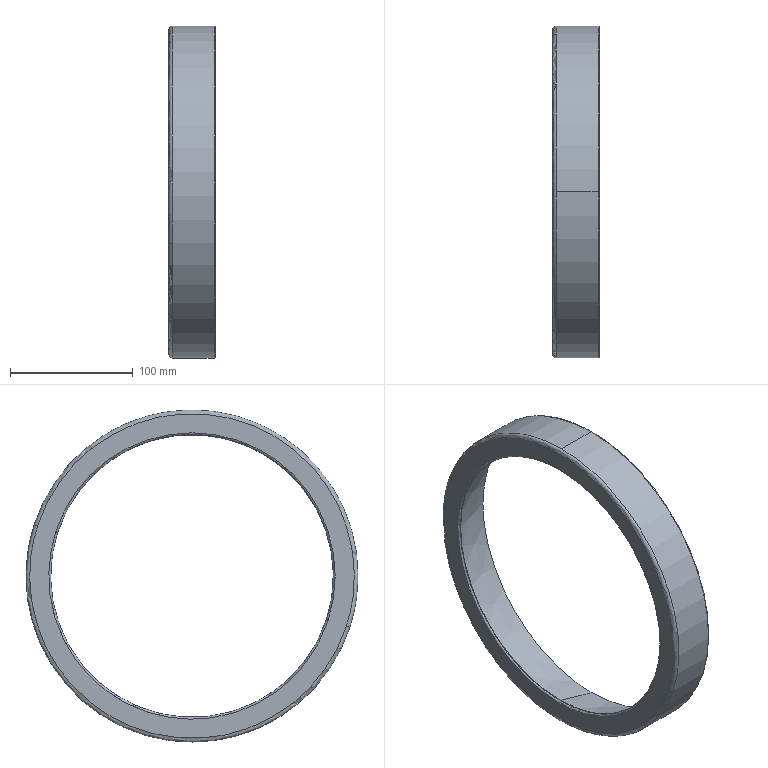Part | SolidWorks | features BaseBody 1 | 1 solid | 14 faces | box 38 x 270 x 270 mm | volume 453986 mm3 | torus 8 | plane 2 | cylinder 2 | cone 2 | commonest cylinder face diameters 270 x2
STEP:
#1=CARTESIAN_POINT('',(0.,-110.751,-35.985));
#2=VERTEX_POINT('',#1);
#3=CARTESIAN_POINT('',(1.5,-109.325,-35.522));
#4=VERTEX_POINT('',#3);
#5=CARTESIAN_POINT('',(1.5,-110.751,-35.985));
#6=DIRECTION('',(0.,0.309,-0.9511));
#7=DIRECTION('',(-1.,0.,0.));
#8=AXIS2_PLACEMENT_3D('',#5,#6,#7);
#9=CIRCLE('',#8,1.5);
#10=EDGE_CURVE('',#2,#4,#9,.T.);
#11=ORIENTED_EDGE('',*,*,#10,.T.);
#12=CARTESIAN_POINT('',(1.5,109.325,35.522));
#13=VERTEX_POINT('',#12);
#14=CARTESIAN_POINT('',(1.5,0.,0.));
#15=DIRECTION('',(1.,0.,0.));
#16=DIRECTION('',(0.,0.,-1.));
#17=AXIS2_PLACEMENT_3D('',#14,#15,#16);
#18=CIRCLE('',#17,114.951);
#19=EDGE_CURVE('',#4,#13,#18,.T.);
#20=ORIENTED_EDGE('',*,*,#19,.T.);
#21=CARTESIAN_POINT('',(0.,110.751,35.985));
#22=VERTEX_POINT('',#21);
#23=CARTESIAN_POINT('',(1.5,110.751,35.985));
#24=DIRECTION('',(0.,-0.309,0.9511));
#25=DIRECTION('',(-1.,0.,0.));
#26=AXIS2_PLACEMENT_3D('',#23,#24,#25);
#27=CIRCLE('',#26,1.5);
#28=EDGE_CURVE('',#22,#13,#27,.T.);
#29=ORIENTED_EDGE('',*,*,#28,.F.);
#30=CARTESIAN_POINT('',(0.,-110.751,-35.985));
#31=CARTESIAN_POINT('',(0.,-108.396,-43.234));
#32=CARTESIAN_POINT('',(0.,-105.327,-50.25));
#33=CARTESIAN_POINT('',(0.,-97.879,-63.55));
#34=CARTESIAN_POINT('',(0.,-93.5,-69.833));
#35=CARTESIAN_POINT('',(0.,-83.6,-81.424));
#36=CARTESIAN_POINT('',(0.,-78.079,-86.732));
#37=CARTESIAN_POINT('',(0.,-66.109,-96.169));
#38=CARTESIAN_POINT('',(0.,-59.659,-100.298));
#39=CARTESIAN_POINT('',(0.,-46.077,-107.219));
#40=CARTESIAN_POINT('',(0.,-38.945,-110.01));
#41=CARTESIAN_POINT('',(0.,-24.274,-114.147));
#42=CARTESIAN_POINT('',(0.,-16.735,-115.494));
#43=CARTESIAN_POINT('',(0.,-1.538,-116.69));
#44=CARTESIAN_POINT('',(0.,6.118,-116.539));
#45=CARTESIAN_POINT('',(0.,21.256,-114.748));
#46=CARTESIAN_POINT('',(0.,28.737,-113.106));
#47=CARTESIAN_POINT('',(0.,43.234,-108.396));
#48=CARTESIAN_POINT('',(0.,50.25,-105.327));
#49=CARTESIAN_POINT('',(0.,63.55,-97.879));
#50=CARTESIAN_POINT('',(0.,69.833,-93.5));
#51=CARTESIAN_POINT('',(0.,81.424,-83.6));
#52=CARTESIAN_POINT('',(0.,86.732,-78.079));
#53=CARTESIAN_POINT('',(0.,96.169,-66.109));
#54=CARTESIAN_POINT('',(0.,100.298,-59.659));
#55=CARTESIAN_POINT('',(0.,107.219,-46.077));
#56=CARTESIAN_POINT('',(0.,110.01,-38.945));
#57=CARTESIAN_POINT('',(0.,114.147,-24.274));
#58=CARTESIAN_POINT('',(0.,115.494,-16.735));
#59=CARTESIAN_POINT('',(0.,116.69,-1.538));
#60=CARTESIAN_POINT('',(0.,116.539,6.118));
#61=CARTESIAN_POINT('',(0.,114.748,21.256));
#62=CARTESIAN_POINT('',(0.,113.106,28.737));
#63=CARTESIAN_POINT('',(0.,110.751,35.985));
#64=B_SPLINE_CURVE_WITH_KNOTS('',3,(#30,#31,#32,#33,#34,#35,#36,#37,#38,#39,#40,#41,#42,#43,#44,#45,#46,#47,#48,#49,#50,#51,#52,#53,#54,#55,#56,#57,#58,#59,#60,#61,#62,#63),.UNSPECIFIED.,.F.,.F.,(4,2,2,2,2,2,2,2,2,2,2,2,2,2,2,2,4),(0.,0.1963,0.3927,0.589,0.7854,0.9817,1.178,1.374,1.571,1.767,1.963,2.16,2.356,2.553,2.749,2.945,3.142),.UNSPECIFIED.);
#65=EDGE_CURVE('',#2,#22,#64,.T.);
#66=ORIENTED_EDGE('',*,*,#65,.F.);
#67=EDGE_LOOP('',(#11,#20,#29,#66));
#68=FACE_OUTER_BOUND('',#67,.T.);
#69=CARTESIAN_POINT('',(1.5,0.,0.));
#70=DIRECTION('',(1.,0.,0.));
#71=DIRECTION('',(0.,-0.309,0.9511));
#72=AXIS2_PLACEMENT_3D('',#69,#70,#71);
#73=TOROIDAL_SURFACE('',#72,116.451,1.5);
#74=ADVANCED_FACE('',(#68),#73,.T.);
#75=ORIENTED_EDGE('',*,*,#28,.T.);
#76=CARTESIAN_POINT('',(1.5,0.,0.));
#77=DIRECTION('',(1.,0.,0.));
#78=DIRECTION('',(0.,0.,-1.));
#79=AXIS2_PLACEMENT_3D('',#76,#77,#78);
#80=CIRCLE('',#79,114.951);
#81=EDGE_CURVE('',#13,#4,#80,.T.);
#82=ORIENTED_EDGE('',*,*,#81,.T.);
#83=ORIENTED_EDGE('',*,*,#10,.F.);
#84=CARTESIAN_POINT('',(0.,0.,0.));
#85=DIRECTION('',(1.,0.,0.));
#86=DIRECTION('',(0.,0.,-1.));
#87=AXIS2_PLACEMENT_3D('',#84,#85,#86);
#88=CIRCLE('',#87,116.451);
#89=EDGE_CURVE('',#22,#2,#88,.T.);
#90=ORIENTED_EDGE('',*,*,#89,.F.);
#91=EDGE_LOOP('',(#75,#82,#83,#90));
#92=FACE_OUTER_BOUND('',#91,.T.);
#93=CARTESIAN_POINT('',(1.5,0.,0.));
#94=DIRECTION('',(1.,0.,0.));
#95=DIRECTION('',(0.,0.309,-0.9511));
#96=AXIS2_PLACEMENT_3D('',#93,#94,#95);
#97=TOROIDAL_SURFACE('',#96,116.451,1.5);
#98=ADVANCED_FACE('',(#92),#97,.T.);
#99=ORIENTED_EDGE('',*,*,#89,.T.);
#100=ORIENTED_EDGE('',*,*,#65,.T.);
#101=EDGE_LOOP('',(#99,#100));
#102=FACE_BOUND('',#101,.T.);
#103=CARTESIAN_POINT('',(0.,125.539,40.79));
#104=VERTEX_POINT('',#103);
#105=CARTESIAN_POINT('',(0.,-125.539,-40.79));
#106=VERTEX_POINT('',#105);
#107=CARTESIAN_POINT('',(0.,125.539,40.79));
#108=CARTESIAN_POINT('',(0.,122.87,49.007));
#109=CARTESIAN_POINT('',(0.,119.391,56.96));
#110=CARTESIAN_POINT('',(0.,110.948,72.036));
#111=CARTESIAN_POINT('',(0.,105.984,79.158));
#112=CARTESIAN_POINT('',(0.,94.763,92.297));
#113=CARTESIAN_POINT('',(0.,88.505,98.313));
#114=CARTESIAN_POINT('',(0.,74.936,109.01));
#115=CARTESIAN_POINT('',(0.,67.624,113.691));
#116=CARTESIAN_POINT('',(0.,52.229,121.535));
#117=CARTESIAN_POINT('',(0.,44.145,124.699));
#118=CARTESIAN_POINT('',(0.,27.515,129.389));
#119=CARTESIAN_POINT('',(0.,18.969,130.915));
#120=CARTESIAN_POINT('',(0.,1.744,132.271));
#121=CARTESIAN_POINT('',(0.,-6.935,132.1));
#122=CARTESIAN_POINT('',(0.,-24.094,130.07));
#123=CARTESIAN_POINT('',(0.,-32.574,128.209));
#124=CARTESIAN_POINT('',(0.,-49.007,122.87));
#125=CARTESIAN_POINT('',(0.,-56.96,119.391));
#126=CARTESIAN_POINT('',(0.,-72.036,110.948));
#127=CARTESIAN_POINT('',(0.,-79.158,105.984));
#128=CARTESIAN_POINT('',(0.,-92.297,94.763));
#129=CARTESIAN_POINT('',(0.,-98.313,88.505));
#130=CARTESIAN_POINT('',(0.,-109.01,74.936));
#131=CARTESIAN_POINT('',(0.,-113.691,67.624));
#132=CARTESIAN_POINT('',(0.,-121.535,52.229));
#133=CARTESIAN_POINT('',(0.,-124.699,44.145));
#134=CARTESIAN_POINT('',(0.,-129.389,27.515));
#135=CARTESIAN_POINT('',(0.,-130.915,18.969));
#136=CARTESIAN_POINT('',(0.,-132.271,1.744));
#137=CARTESIAN_POINT('',(0.,-132.1,-6.935));
#138=CARTESIAN_POINT('',(0.,-130.07,-24.094));
#139=CARTESIAN_POINT('',(0.,-128.209,-32.574));
#140=CARTESIAN_POINT('',(0.,-125.539,-40.79));
#141=B_SPLINE_CURVE_WITH_KNOTS('',3,(#107,#108,#109,#110,#111,#112,#113,#114,#115,#116,#117,#118,#119,#120,#121,#122,#123,#124,#125,#126,#127,#128,#129,#130,#131,#132,#133,#134,#135,#136,#137,#138,#139,#140),.UNSPECIFIED.,.F.,.F.,(4,2,2,2,2,2,2,2,2,2,2,2,2,2,2,2,4),(0.,0.1963,0.3927,0.589,0.7854,0.9817,1.178,1.374,1.571,1.767,1.963,2.16,2.356,2.553,2.749,2.945,3.142),.UNSPECIFIED.);
#142=EDGE_CURVE('',#104,#106,#141,.T.);
#143=ORIENTED_EDGE('',*,*,#142,.F.);
#144=CARTESIAN_POINT('',(0.,-125.539,-40.79));
#145=CARTESIAN_POINT('',(0.,-122.87,-49.007));
#146=CARTESIAN_POINT('',(0.,-119.391,-56.96));
#147=CARTESIAN_POINT('',(0.,-110.948,-72.036));
#148=CARTESIAN_POINT('',(0.,-105.984,-79.158));
#149=CARTESIAN_POINT('',(0.,-94.763,-92.297));
#150=CARTESIAN_POINT('',(0.,-88.505,-98.313));
#151=CARTESIAN_POINT('',(0.,-74.936,-109.01));
#152=CARTESIAN_POINT('',(0.,-67.624,-113.691));
#153=CARTESIAN_POINT('',(0.,-52.229,-121.535));
#154=CARTESIAN_POINT('',(0.,-44.145,-124.699));
#155=CARTESIAN_POINT('',(0.,-27.515,-129.389));
#156=CARTESIAN_POINT('',(0.,-18.969,-130.915));
#157=CARTESIAN_POINT('',(0.,-1.744,-132.271));
#158=CARTESIAN_POINT('',(0.,6.935,-132.1));
#159=CARTESIAN_POINT('',(0.,24.094,-130.07));
#160=CARTESIAN_POINT('',(0.,32.574,-128.209));
#161=CARTESIAN_POINT('',(0.,49.007,-122.87));
#162=CARTESIAN_POINT('',(0.,56.96,-119.391));
#163=CARTESIAN_POINT('',(0.,72.036,-110.948));
#164=CARTESIAN_POINT('',(0.,79.158,-105.984));
#165=CARTESIAN_POINT('',(0.,92.297,-94.763));
#166=CARTESIAN_POINT('',(0.,98.313,-88.505));
#167=CARTESIAN_POINT('',(0.,109.01,-74.936));
#168=CARTESIAN_POINT('',(0.,113.691,-67.624));
#169=CARTESIAN_POINT('',(0.,121.535,-52.229));
#170=CARTESIAN_POINT('',(0.,124.699,-44.145));
#171=CARTESIAN_POINT('',(0.,129.389,-27.515));
#172=CARTESIAN_POINT('',(0.,130.915,-18.969));
#173=CARTESIAN_POINT('',(0.,132.271,-1.744));
#174=CARTESIAN_POINT('',(0.,132.1,6.935));
#175=CARTESIAN_POINT('',(0.,130.07,24.094));
#176=CARTESIAN_POINT('',(0.,128.209,32.574));
#177=CARTESIAN_POINT('',(0.,125.539,40.79));
#178=B_SPLINE_CURVE_WITH_KNOTS('',3,(#144,#145,#146,#147,#148,#149,#150,#151,#152,#153,#154,#155,#156,#157,#158,#159,#160,#161,#162,#163,#164,#165,#166,#167,#168,#169,#170,#171,#172,#173,#174,#175,#176,#177),.UNSPECIFIED.,.F.,.F.,(4,2,2,2,2,2,2,2,2,2,2,2,2,2,2,2,4),(0.,0.1963,0.3927,0.589,0.7854,0.9817,1.178,1.374,1.571,1.767,1.963,2.16,2.356,2.553,2.749,2.945,3.142),.UNSPECIFIED.);
#179=EDGE_CURVE('',#106,#104,#178,.T.);
#180=ORIENTED_EDGE('',*,*,#179,.F.);
#181=EDGE_LOOP('',(#143,#180));
#182=FACE_OUTER_BOUND('',#181,.T.);
#183=CARTESIAN_POINT('',(0.,132.,0.));
#184=DIRECTION('',(-1.,0.,0.));
#185=DIRECTION('',(0.,0.,1.));
#186=AXIS2_PLACEMENT_3D('',#183,#184,#185);
#187=PLANE('',#186);
#188=ADVANCED_FACE('',(#102,#182),#187,.T.);
#189=CARTESIAN_POINT('',(3.,-128.393,-41.717));
#190=VERTEX_POINT('',#189);
#191=CARTESIAN_POINT('',(3.,-125.539,-40.79));
#192=DIRECTION('',(0.,0.309,-0.9511));
#193=DIRECTION('',(0.,-0.9511,-0.309));
#194=AXIS2_PLACEMENT_3D('',#191,#192,#193);
#195=CIRCLE('',#194,3.);
#196=EDGE_CURVE('',#190,#106,#195,.T.);
#197=ORIENTED_EDGE('',*,*,#196,.T.);
#198=ORIENTED_EDGE('',*,*,#179,.T.);
#199=CARTESIAN_POINT('',(3.,128.393,41.717));
#200=VERTEX_POINT('',#199);
#201=CARTESIAN_POINT('',(3.,125.539,40.79));
#202=DIRECTION('',(0.,-0.309,0.9511));
#203=DIRECTION('',(0.,0.9511,0.309));
#204=AXIS2_PLACEMENT_3D('',#201,#202,#203);
#205=CIRCLE('',#204,3.);
#206=EDGE_CURVE('',#200,#104,#205,.T.);
#207=ORIENTED_EDGE('',*,*,#206,.F.);
#208=CARTESIAN_POINT('',(3.,0.,-135.));
#209=VERTEX_POINT('',#208);
#210=CARTESIAN_POINT('',(3.,0.,0.));
#211=DIRECTION('',(1.,0.,0.));
#212=DIRECTION('',(0.,0.,-1.));
#213=AXIS2_PLACEMENT_3D('',#210,#211,#212);
#214=CIRCLE('',#213,135.);
#215=EDGE_CURVE('',#209,#200,#214,.T.);
#216=ORIENTED_EDGE('',*,*,#215,.F.);
#217=CARTESIAN_POINT('',(3.,0.,0.));
#218=DIRECTION('',(1.,0.,0.));
#219=DIRECTION('',(0.,0.,-1.));
#220=AXIS2_PLACEMENT_3D('',#217,#218,#219);
#221=CIRCLE('',#220,135.);
#222=EDGE_CURVE('',#190,#209,#221,.T.);
#223=ORIENTED_EDGE('',*,*,#222,.F.);
#224=EDGE_LOOP('',(#197,#198,#207,#216,#223));
#225=FACE_OUTER_BOUND('',#224,.T.);
#226=CARTESIAN_POINT('',(3.,0.,0.));
#227=DIRECTION('',(1.,0.,0.));
#228=DIRECTION('',(0.,-0.309,0.9511));
#229=AXIS2_PLACEMENT_3D('',#226,#227,#228);
#230=TOROIDAL_SURFACE('',#229,132.,3.);
#231=ADVANCED_FACE('',(#225),#230,.T.);
#232=CARTESIAN_POINT('',(3.,0.,135.));
#233=VERTEX_POINT('',#232);
#234=CARTESIAN_POINT('',(37.,0.,135.));
#235=VERTEX_POINT('',#234);
#236=CARTESIAN_POINT('',(3.,0.,135.));
#237=DIRECTION('',(1.,0.,0.));
#238=VECTOR('',#237,1000.);
#239=LINE('',#236,#238);
#240=EDGE_CURVE('',#233,#235,#239,.T.);
#241=ORIENTED_EDGE('',*,*,#240,.F.);
#242=CARTESIAN_POINT('',(3.,0.,0.));
#243=DIRECTION('',(1.,0.,0.));
#244=DIRECTION('',(0.,0.,-1.));
#245=AXIS2_PLACEMENT_3D('',#242,#243,#244);
#246=CIRCLE('',#245,135.);
#247=EDGE_CURVE('',#233,#190,#246,.T.);
#248=ORIENTED_EDGE('',*,*,#247,.T.);
#249=ORIENTED_EDGE('',*,*,#222,.T.);
#250=CARTESIAN_POINT('',(37.,0.,-135.));
#251=VERTEX_POINT('',#250);
#252=CARTESIAN_POINT('',(3.,0.,-135.));
#253=DIRECTION('',(1.,0.,0.));
#254=VECTOR('',#253,1000.);
#255=LINE('',#252,#254);
#256=EDGE_CURVE('',#209,#251,#255,.T.);
#257=ORIENTED_EDGE('',*,*,#256,.T.);
#258=CARTESIAN_POINT('',(37.,-128.393,-41.717));
#259=VERTEX_POINT('',#258);
#260=CARTESIAN_POINT('',(37.,0.,0.));
#261=DIRECTION('',(1.,0.,0.));
#262=DIRECTION('',(0.,0.,-1.));
#263=AXIS2_PLACEMENT_3D('',#260,#261,#262);
#264=CIRCLE('',#263,135.);
#265=EDGE_CURVE('',#259,#251,#264,.T.);
#266=ORIENTED_EDGE('',*,*,#265,.F.);
#267=CARTESIAN_POINT('',(37.,0.,0.));
#268=DIRECTION('',(1.,0.,0.));
#269=DIRECTION('',(0.,0.,-1.));
#270=AXIS2_PLACEMENT_3D('',#267,#268,#269);
#271=CIRCLE('',#270,135.);
#272=EDGE_CURVE('',#235,#259,#271,.T.);
#273=ORIENTED_EDGE('',*,*,#272,.F.);
#274=EDGE_LOOP('',(#241,#248,#249,#257,#266,#273));
#275=FACE_OUTER_BOUND('',#274,.T.);
#276=CARTESIAN_POINT('',(38.,0.,0.));
#277=DIRECTION('',(1.,0.,0.));
#278=DIRECTION('',(0.,1.,0.));
#279=AXIS2_PLACEMENT_3D('',#276,#277,#278);
#280=CYLINDRICAL_SURFACE('',#279,135.);
#281=ADVANCED_FACE('',(#275),#280,.T.);
#282=CARTESIAN_POINT('',(38.,-127.442,-41.408));
#283=VERTEX_POINT('',#282);
#284=CARTESIAN_POINT('',(37.,-127.442,-41.408));
#285=DIRECTION('',(0.,0.309,-0.9511));
#286=DIRECTION('',(1.,0.,0.));
#287=AXIS2_PLACEMENT_3D('',#284,#285,#286);
#288=CIRCLE('',#287,1.);
#289=EDGE_CURVE('',#283,#259,#288,.T.);
#290=ORIENTED_EDGE('',*,*,#289,.F.);
#291=CARTESIAN_POINT('',(38.,127.442,41.408));
#292=VERTEX_POINT('',#291);
#293=CARTESIAN_POINT('',(38.,0.,0.));
#294=DIRECTION('',(1.,0.,0.));
#295=DIRECTION('',(0.,0.,-1.));
#296=AXIS2_PLACEMENT_3D('',#293,#294,#295);
#297=CIRCLE('',#296,134.);
#298=EDGE_CURVE('',#292,#283,#297,.T.);
#299=ORIENTED_EDGE('',*,*,#298,.F.);
#300=CARTESIAN_POINT('',(37.,128.393,41.717));
#301=VERTEX_POINT('',#300);
#302=CARTESIAN_POINT('',(37.,127.442,41.408));
#303=DIRECTION('',(0.,-0.309,0.9511));
#304=DIRECTION('',(1.,0.,0.));
#305=AXIS2_PLACEMENT_3D('',#302,#303,#304);
#306=CIRCLE('',#305,1.);
#307=EDGE_CURVE('',#292,#301,#306,.T.);
#308=ORIENTED_EDGE('',*,*,#307,.T.);
#309=CARTESIAN_POINT('',(37.,0.,0.));
#310=DIRECTION('',(1.,0.,0.));
#311=DIRECTION('',(0.,0.,-1.));
#312=AXIS2_PLACEMENT_3D('',#309,#310,#311);
#313=CIRCLE('',#312,135.);
#314=EDGE_CURVE('',#301,#235,#313,.T.);
#315=ORIENTED_EDGE('',*,*,#314,.T.);
#316=ORIENTED_EDGE('',*,*,#272,.T.);
#317=EDGE_LOOP('',(#290,#299,#308,#315,#316));
#318=FACE_OUTER_BOUND('',#317,.T.);
#319=CARTESIAN_POINT('',(37.,0.,0.));
#320=DIRECTION('',(1.,0.,0.));
#321=DIRECTION('',(0.,0.309,-0.9511));
#322=AXIS2_PLACEMENT_3D('',#319,#320,#321);
#323=TOROIDAL_SURFACE('',#322,134.,1.);
#324=ADVANCED_FACE('',(#318),#323,.T.);
#325=ORIENTED_EDGE('',*,*,#240,.T.);
#326=ORIENTED_EDGE('',*,*,#314,.F.);
#327=CARTESIAN_POINT('',(37.,0.,0.));
#328=DIRECTION('',(1.,0.,0.));
#329=DIRECTION('',(0.,0.,-1.));
#330=AXIS2_PLACEMENT_3D('',#327,#328,#329);
#331=CIRCLE('',#330,135.);
#332=EDGE_CURVE('',#251,#301,#331,.T.);
#333=ORIENTED_EDGE('',*,*,#332,.F.);
#334=ORIENTED_EDGE('',*,*,#256,.F.);
#335=ORIENTED_EDGE('',*,*,#215,.T.);
#336=CARTESIAN_POINT('',(3.,0.,0.));
#337=DIRECTION('',(1.,0.,0.));
#338=DIRECTION('',(0.,0.,-1.));
#339=AXIS2_PLACEMENT_3D('',#336,#337,#338);
#340=CIRCLE('',#339,135.);
#341=EDGE_CURVE('',#200,#233,#340,.T.);
#342=ORIENTED_EDGE('',*,*,#341,.T.);
#343=EDGE_LOOP('',(#325,#326,#333,#334,#335,#342));
#344=FACE_OUTER_BOUND('',#343,.T.);
#345=CARTESIAN_POINT('',(38.,0.,0.));
#346=DIRECTION('',(1.,0.,0.));
#347=DIRECTION('',(0.,-1.,0.));
#348=AXIS2_PLACEMENT_3D('',#345,#346,#347);
#349=CYLINDRICAL_SURFACE('',#348,135.);
#350=ADVANCED_FACE('',(#344),#349,.T.);
#351=ORIENTED_EDGE('',*,*,#196,.F.);
#352=ORIENTED_EDGE('',*,*,#247,.F.);
#353=ORIENTED_EDGE('',*,*,#341,.F.);
#354=ORIENTED_EDGE('',*,*,#206,.T.);
#355=ORIENTED_EDGE('',*,*,#142,.T.);
#356=EDGE_LOOP('',(#351,#352,#353,#354,#355));
#357=FACE_OUTER_BOUND('',#356,.T.);
#358=CARTESIAN_POINT('',(3.,0.,0.));
#359=DIRECTION('',(1.,0.,0.));
#360=DIRECTION('',(0.,0.309,-0.9511));
#361=AXIS2_PLACEMENT_3D('',#358,#359,#360);
#362=TOROIDAL_SURFACE('',#361,132.,3.);
#363=ADVANCED_FACE('',(#357),#362,.T.);
#364=ORIENTED_EDGE('',*,*,#289,.T.);
#365=ORIENTED_EDGE('',*,*,#265,.T.);
#366=ORIENTED_EDGE('',*,*,#332,.T.);
#367=ORIENTED_EDGE('',*,*,#307,.F.);
#368=CARTESIAN_POINT('',(38.,-127.442,-41.408));
#369=CARTESIAN_POINT('',(38.,-124.731,-49.749));
#370=CARTESIAN_POINT('',(38.,-121.2,-57.823));
#371=CARTESIAN_POINT('',(38.,-112.629,-73.127));
#372=CARTESIAN_POINT('',(38.,-107.59,-80.357));
#373=CARTESIAN_POINT('',(38.,-96.199,-93.695));
#374=CARTESIAN_POINT('',(38.,-89.846,-99.803));
#375=CARTESIAN_POINT('',(38.,-76.071,-110.662));
#376=CARTESIAN_POINT('',(38.,-68.649,-115.413));
#377=CARTESIAN_POINT('',(38.,-53.02,-123.376));
#378=CARTESIAN_POINT('',(38.,-44.814,-126.588));
#379=CARTESIAN_POINT('',(38.,-27.932,-131.35));
#380=CARTESIAN_POINT('',(38.,-19.257,-132.899));
#381=CARTESIAN_POINT('',(38.,-1.77,-134.275));
#382=CARTESIAN_POINT('',(38.,7.041,-134.102));
#383=CARTESIAN_POINT('',(38.,24.459,-132.04));
#384=CARTESIAN_POINT('',(38.,33.067,-130.152));
#385=CARTESIAN_POINT('',(38.,49.749,-124.731));
#386=CARTESIAN_POINT('',(38.,57.823,-121.2));
#387=CARTESIAN_POINT('',(38.,73.127,-112.629));
#388=CARTESIAN_POINT('',(38.,80.357,-107.59));
#389=CARTESIAN_POINT('',(38.,93.695,-96.199));
#390=CARTESIAN_POINT('',(38.,99.803,-89.846));
#391=CARTESIAN_POINT('',(38.,110.662,-76.071));
#392=CARTESIAN_POINT('',(38.,115.413,-68.649));
#393=CARTESIAN_POINT('',(38.,123.376,-53.02));
#394=CARTESIAN_POINT('',(38.,126.588,-44.814));
#395=CARTESIAN_POINT('',(38.,131.35,-27.932));
#396=CARTESIAN_POINT('',(38.,132.899,-19.257));
#397=CARTESIAN_POINT('',(38.,134.275,-1.77));
#398=CARTESIAN_POINT('',(38.,134.102,7.041));
#399=CARTESIAN_POINT('',(38.,132.04,24.459));
#400=CARTESIAN_POINT('',(38.,130.152,33.067));
#401=CARTESIAN_POINT('',(38.,127.442,41.408));
#402=B_SPLINE_CURVE_WITH_KNOTS('',3,(#368,#369,#370,#371,#372,#373,#374,#375,#376,#377,#378,#379,#380,#381,#382,#383,#384,#385,#386,#387,#388,#389,#390,#391,#392,#393,#394,#395,#396,#397,#398,#399,#400,#401),.UNSPECIFIED.,.F.,.F.,(4,2,2,2,2,2,2,2,2,2,2,2,2,2,2,2,4),(0.,0.1963,0.3927,0.589,0.7854,0.9817,1.178,1.374,1.571,1.767,1.963,2.16,2.356,2.553,2.749,2.945,3.142),.UNSPECIFIED.);
#403=EDGE_CURVE('',#283,#292,#402,.T.);
#404=ORIENTED_EDGE('',*,*,#403,.F.);
#405=EDGE_LOOP('',(#364,#365,#366,#367,#404));
#406=FACE_OUTER_BOUND('',#405,.T.);
#407=CARTESIAN_POINT('',(37.,0.,0.));
#408=DIRECTION('',(1.,0.,0.));
#409=DIRECTION('',(0.,-0.309,0.9511));
#410=AXIS2_PLACEMENT_3D('',#407,#408,#409);
#411=TOROIDAL_SURFACE('',#410,134.,1.);
#412=ADVANCED_FACE('',(#406),#411,.T.);
#413=ORIENTED_EDGE('',*,*,#298,.T.);
#414=ORIENTED_EDGE('',*,*,#403,.T.);
#415=EDGE_LOOP('',(#413,#414));
#416=FACE_OUTER_BOUND('',#415,.T.);
#417=CARTESIAN_POINT('',(38.,0.,125.474));
#418=VERTEX_POINT('',#417);
#419=CARTESIAN_POINT('',(38.,0.,-125.474));
#420=VERTEX_POINT('',#419);
#421=CARTESIAN_POINT('',(38.,0.,0.));
#422=DIRECTION('',(1.,0.,0.));
#423=DIRECTION('',(0.,0.,-1.));
#424=AXIS2_PLACEMENT_3D('',#421,#422,#423);
#425=CIRCLE('',#424,125.474);
#426=EDGE_CURVE('',#418,#420,#425,.T.);
#427=ORIENTED_EDGE('',*,*,#426,.F.);
#428=CARTESIAN_POINT('',(38.,0.,0.));
#429=DIRECTION('',(1.,0.,0.));
#430=DIRECTION('',(0.,0.,-1.));
#431=AXIS2_PLACEMENT_3D('',#428,#429,#430);
#432=CIRCLE('',#431,125.474);
#433=EDGE_CURVE('',#420,#418,#432,.T.);
#434=ORIENTED_EDGE('',*,*,#433,.F.);
#435=EDGE_LOOP('',(#427,#434));
#436=FACE_BOUND('',#435,.T.);
#437=CARTESIAN_POINT('',(38.,125.474,0.));
#438=DIRECTION('',(1.,0.,0.));
#439=DIRECTION('',(0.,0.,-1.));
#440=AXIS2_PLACEMENT_3D('',#437,#438,#439);
#441=PLANE('',#440);
#442=ADVANCED_FACE('',(#416,#436),#441,.T.);
#443=CARTESIAN_POINT('',(1.918,0.,115.01));
#444=VERTEX_POINT('',#443);
#445=CARTESIAN_POINT('',(1.918,0.,115.01));
#446=DIRECTION('',(0.9604,0.,0.2785));
#447=VECTOR('',#446,1000.);
#448=LINE('',#445,#447);
#449=EDGE_CURVE('',#444,#418,#448,.T.);
#450=ORIENTED_EDGE('',*,*,#449,.F.);
#451=CARTESIAN_POINT('',(1.918,109.381,35.54));
#452=VERTEX_POINT('',#451);
#453=CARTESIAN_POINT('',(1.918,0.,0.));
#454=DIRECTION('',(1.,0.,0.));
#455=DIRECTION('',(0.,0.,-1.));
#456=AXIS2_PLACEMENT_3D('',#453,#454,#455);
#457=CIRCLE('',#456,115.01);
#458=EDGE_CURVE('',#452,#444,#457,.T.);
#459=ORIENTED_EDGE('',*,*,#458,.F.);
#460=CARTESIAN_POINT('',(1.918,0.,-115.01));
#461=VERTEX_POINT('',#460);
#462=CARTESIAN_POINT('',(1.918,0.,0.));
#463=DIRECTION('',(1.,0.,0.));
#464=DIRECTION('',(0.,0.,-1.));
#465=AXIS2_PLACEMENT_3D('',#462,#463,#464);
#466=CIRCLE('',#465,115.01);
#467=EDGE_CURVE('',#461,#452,#466,.T.);
#468=ORIENTED_EDGE('',*,*,#467,.F.);
#469=CARTESIAN_POINT('',(1.918,0.,-115.01));
#470=DIRECTION('',(0.9604,0.,-0.2785));
#471=VECTOR('',#470,1000.);
#472=LINE('',#469,#471);
#473=EDGE_CURVE('',#461,#420,#472,.T.);
#474=ORIENTED_EDGE('',*,*,#473,.T.);
#475=ORIENTED_EDGE('',*,*,#433,.T.);
#476=EDGE_LOOP('',(#450,#459,#468,#474,#475));
#477=FACE_OUTER_BOUND('',#476,.T.);
#478=CARTESIAN_POINT('',(1.918,0.,0.));
#479=DIRECTION('',(1.,0.,0.));
#480=DIRECTION('',(0.,-1.,0.));
#481=AXIS2_PLACEMENT_3D('',#478,#479,#480);
#482=CONICAL_SURFACE('',#481,115.01,0.2823);
#483=ADVANCED_FACE('',(#477),#482,.F.);
#484=ORIENTED_EDGE('',*,*,#449,.T.);
#485=ORIENTED_EDGE('',*,*,#426,.T.);
#486=ORIENTED_EDGE('',*,*,#473,.F.);
#487=CARTESIAN_POINT('',(1.918,-109.381,-35.54));
#488=VERTEX_POINT('',#487);
#489=CARTESIAN_POINT('',(1.918,0.,0.));
#490=DIRECTION('',(1.,0.,0.));
#491=DIRECTION('',(0.,0.,-1.));
#492=AXIS2_PLACEMENT_3D('',#489,#490,#491);
#493=CIRCLE('',#492,115.01);
#494=EDGE_CURVE('',#488,#461,#493,.T.);
#495=ORIENTED_EDGE('',*,*,#494,.F.);
#496=CARTESIAN_POINT('',(1.918,0.,0.));
#497=DIRECTION('',(1.,0.,0.));
#498=DIRECTION('',(0.,0.,-1.));
#499=AXIS2_PLACEMENT_3D('',#496,#497,#498);
#500=CIRCLE('',#499,115.01);
#501=EDGE_CURVE('',#444,#488,#500,.T.);
#502=ORIENTED_EDGE('',*,*,#501,.F.);
#503=EDGE_LOOP('',(#484,#485,#486,#495,#502));
#504=FACE_OUTER_BOUND('',#503,.T.);
#505=CARTESIAN_POINT('',(1.918,0.,0.));
#506=DIRECTION('',(1.,0.,0.));
#507=DIRECTION('',(0.,1.,0.));
#508=AXIS2_PLACEMENT_3D('',#505,#506,#507);
#509=CONICAL_SURFACE('',#508,115.01,0.2823);
#510=ADVANCED_FACE('',(#504),#509,.F.);
#511=ORIENTED_EDGE('',*,*,#81,.F.);
#512=CARTESIAN_POINT('',(1.5,110.751,35.985));
#513=DIRECTION('',(0.,-0.309,0.9511));
#514=DIRECTION('',(-1.,0.,0.));
#515=AXIS2_PLACEMENT_3D('',#512,#513,#514);
#516=CIRCLE('',#515,1.5);
#517=EDGE_CURVE('',#13,#452,#516,.T.);
#518=ORIENTED_EDGE('',*,*,#517,.T.);
#519=ORIENTED_EDGE('',*,*,#458,.T.);
#520=ORIENTED_EDGE('',*,*,#501,.T.);
#521=CARTESIAN_POINT('',(1.5,-110.751,-35.985));
#522=DIRECTION('',(0.,0.309,-0.9511));
#523=DIRECTION('',(-1.,0.,0.));
#524=AXIS2_PLACEMENT_3D('',#521,#522,#523);
#525=CIRCLE('',#524,1.5);
#526=EDGE_CURVE('',#4,#488,#525,.T.);
#527=ORIENTED_EDGE('',*,*,#526,.F.);
#528=EDGE_LOOP('',(#511,#518,#519,#520,#527));
#529=FACE_OUTER_BOUND('',#528,.T.);
#530=CARTESIAN_POINT('',(1.5,0.,0.));
#531=DIRECTION('',(1.,0.,0.));
#532=DIRECTION('',(0.,0.309,-0.9511));
#533=AXIS2_PLACEMENT_3D('',#530,#531,#532);
#534=TOROIDAL_SURFACE('',#533,116.451,1.5);
#535=ADVANCED_FACE('',(#529),#534,.T.);
#536=ORIENTED_EDGE('',*,*,#19,.F.);
#537=ORIENTED_EDGE('',*,*,#526,.T.);
#538=ORIENTED_EDGE('',*,*,#494,.T.);
#539=ORIENTED_EDGE('',*,*,#467,.T.);
#540=ORIENTED_EDGE('',*,*,#517,.F.);
#541=EDGE_LOOP('',(#536,#537,#538,#539,#540));
#542=FACE_OUTER_BOUND('',#541,.T.);
#543=CARTESIAN_POINT('',(1.5,0.,0.));
#544=DIRECTION('',(1.,0.,0.));
#545=DIRECTION('',(0.,-0.309,0.9511));
#546=AXIS2_PLACEMENT_3D('',#543,#544,#545);
#547=TOROIDAL_SURFACE('',#546,116.451,1.5);
#548=ADVANCED_FACE('',(#542),#547,.T.);
#549=CLOSED_SHELL('',(#74,#98,#188,#231,#281,#324,#350,#363,#412,#442,#483,#510,#535,#548));
#550=MANIFOLD_SOLID_BREP('',#549);
#551=CARTESIAN_POINT('',(0.,0.,0.));
#552=DIRECTION('',(0.,0.,1.));
#553=DIRECTION('',(1.,0.,0.));
#554=AXIS2_PLACEMENT_3D('',#551,#552,#553);
#555=(LENGTH_UNIT()NAMED_UNIT(*)SI_UNIT(.MILLI.,.METRE.));
#556=UNCERTAINTY_MEASURE_WITH_UNIT(LENGTH_MEASURE(0.00001),#555,'','');
#557=(NAMED_UNIT(*)PLANE_ANGLE_UNIT()SI_UNIT($,.RADIAN.));
#558=(NAMED_UNIT(*)SI_UNIT($,.STERADIAN.)SOLID_ANGLE_UNIT());
#559=(GEOMETRIC_REPRESENTATION_CONTEXT(3)GLOBAL_UNCERTAINTY_ASSIGNED_CONTEXT((#556))GLOBAL_UNIT_ASSIGNED_CONTEXT((#555,#557,#558))REPRESENTATION_CONTEXT('',''));
#560=ADVANCED_BREP_SHAPE_REPRESENTATION('',(#550,#554),#559);